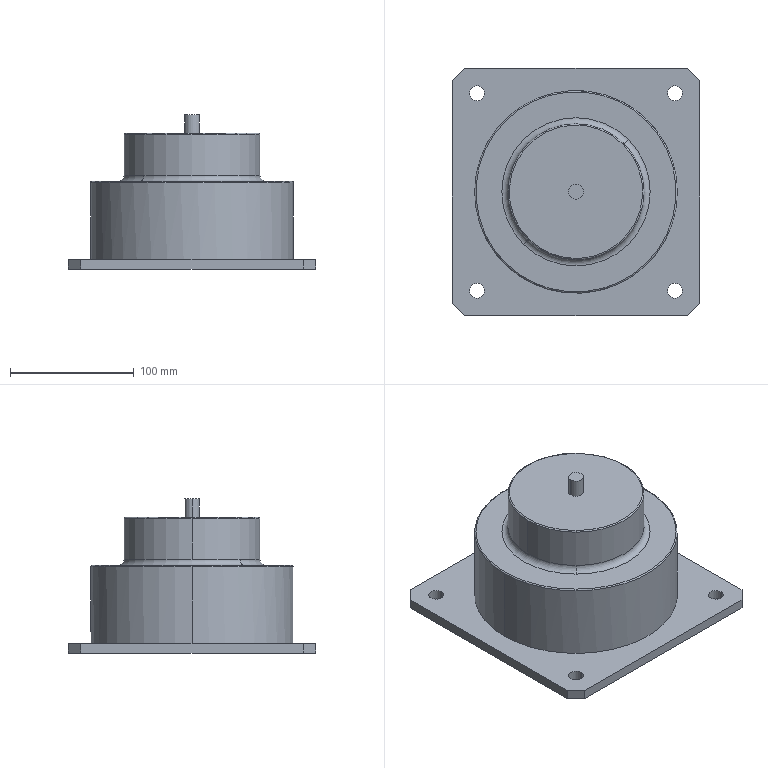Part | STEP file | ASND-0110-E63-HLTP01JSC-700 SA | 1 solid | 33 faces | box 200 x 200 x 125 mm | volume 2019631 mm3 | cylinder 14 | plane 13 | torus 6 | commonest cylinder face diameters 12 x10 110 x2 164 x2